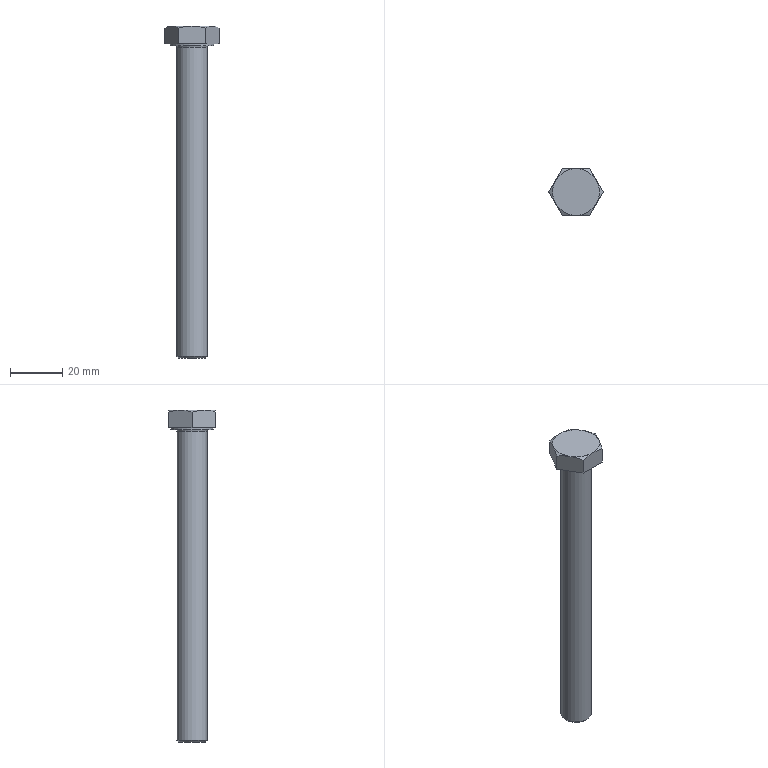Part | NX | features SKETCH 4, EXTRUDE 3, META 3, DATUM_CSYS 2, BLEND 1, CHAMFER 1, DATUM_PLANE 1, LINE 1, SWP104 1, SYMBOLIC_THREAD 1, THREADS 1 | 1 solid | 20 faces | box 20.785 x 18 x 127.5 mm | volume 15029 mm3 | plane 10 | cone 7 | cylinder 2 | torus 1 | commonest cylinder face diameters 11.732 x1 16.63 x1
STEP:
#1=CARTESIAN_POINT('',(5.196,-9.,6.696));
#2=VERTEX_POINT('',#1);
#3=CARTESIAN_POINT('',(7.794,-4.5,7.5));
#4=VERTEX_POINT('',#3);
#5=CARTESIAN_POINT('',(5.196,-9.,6.696));
#6=CARTESIAN_POINT('',(6.046,-7.528,7.187));
#7=CARTESIAN_POINT('',(6.909,-6.033,7.5));
#8=CARTESIAN_POINT('',(7.794,-4.5,7.5));
#9=B_SPLINE_CURVE_WITH_KNOTS('',3,(#5,#6,#7,#8),.UNSPECIFIED.,.F.,.F.,(4,4),(0.000000238,0.005258),.UNSPECIFIED.);
#10=EDGE_CURVE('',#2,#4,#9,.T.);
#11=ORIENTED_EDGE('',*,*,#10,.F.);
#12=CARTESIAN_POINT('',(5.196,-9.,0.6));
#13=VERTEX_POINT('',#12);
#14=CARTESIAN_POINT('',(5.196,-9.,7.5));
#15=DIRECTION('',(0.,0.,-1.));
#16=VECTOR('',#15,1000.);
#17=LINE('',#14,#16);
#18=EDGE_CURVE('',#2,#13,#17,.T.);
#19=ORIENTED_EDGE('',*,*,#18,.T.);
#20=CARTESIAN_POINT('',(10.392,0.,0.6));
#21=VERTEX_POINT('',#20);
#22=CARTESIAN_POINT('',(5.196,-9.,0.6));
#23=DIRECTION('',(0.5,0.866,0.));
#24=VECTOR('',#23,1000.);
#25=LINE('',#22,#24);
#26=EDGE_CURVE('',#13,#21,#25,.T.);
#27=ORIENTED_EDGE('',*,*,#26,.T.);
#28=CARTESIAN_POINT('',(10.392,0.,6.696));
#29=VERTEX_POINT('',#28);
#30=CARTESIAN_POINT('',(10.392,0.,7.5));
#31=DIRECTION('',(0.,0.,-1.));
#32=VECTOR('',#31,1000.);
#33=LINE('',#30,#32);
#34=EDGE_CURVE('',#29,#21,#33,.T.);
#35=ORIENTED_EDGE('',*,*,#34,.F.);
#36=CARTESIAN_POINT('',(7.794,-4.5,7.5));
#37=CARTESIAN_POINT('',(8.676,-2.972,7.5));
#38=CARTESIAN_POINT('',(9.544,-1.469,7.186));
#39=CARTESIAN_POINT('',(10.392,0.,6.696));
#40=B_SPLINE_CURVE_WITH_KNOTS('',3,(#36,#37,#38,#39),.UNSPECIFIED.,.F.,.F.,(4,4),(0.005258,0.0105),.UNSPECIFIED.);
#41=EDGE_CURVE('',#4,#29,#40,.T.);
#42=ORIENTED_EDGE('',*,*,#41,.F.);
#43=EDGE_LOOP('',(#11,#19,#27,#35,#42));
#44=FACE_BOUND('',#43,.T.);
#45=CARTESIAN_POINT('',(5.196,-9.,7.5));
#46=DIRECTION('',(-0.866,0.5,0.));
#47=DIRECTION('',(-0.5,-0.866,0.));
#48=AXIS2_PLACEMENT_3D('',#45,#46,#47);
#49=PLANE('',#48);
#50=ADVANCED_FACE('',(#44),#49,.F.);
#51=CARTESIAN_POINT('',(7.794,4.5,7.5));
#52=VERTEX_POINT('',#51);
#53=CARTESIAN_POINT('',(10.392,0.,6.696));
#54=CARTESIAN_POINT('',(9.542,1.472,7.187));
#55=CARTESIAN_POINT('',(8.679,2.967,7.5));
#56=CARTESIAN_POINT('',(7.794,4.5,7.5));
#57=B_SPLINE_CURVE_WITH_KNOTS('',3,(#53,#54,#55,#56),.UNSPECIFIED.,.F.,.F.,(4,4),(0.000000238,0.005258),.UNSPECIFIED.);
#58=EDGE_CURVE('',#29,#52,#57,.T.);
#59=ORIENTED_EDGE('',*,*,#58,.F.);
#60=ORIENTED_EDGE('',*,*,#34,.T.);
#61=CARTESIAN_POINT('',(5.196,9.,0.6));
#62=VERTEX_POINT('',#61);
#63=CARTESIAN_POINT('',(10.392,0.,0.6));
#64=DIRECTION('',(-0.5,0.866,0.));
#65=VECTOR('',#64,1000.);
#66=LINE('',#63,#65);
#67=EDGE_CURVE('',#21,#62,#66,.T.);
#68=ORIENTED_EDGE('',*,*,#67,.T.);
#69=CARTESIAN_POINT('',(5.196,9.,6.696));
#70=VERTEX_POINT('',#69);
#71=CARTESIAN_POINT('',(5.196,9.,7.5));
#72=DIRECTION('',(0.,0.,-1.));
#73=VECTOR('',#72,1000.);
#74=LINE('',#71,#73);
#75=EDGE_CURVE('',#70,#62,#74,.T.);
#76=ORIENTED_EDGE('',*,*,#75,.F.);
#77=CARTESIAN_POINT('',(7.794,4.5,7.5));
#78=CARTESIAN_POINT('',(6.912,6.028,7.5));
#79=CARTESIAN_POINT('',(6.044,7.531,7.186));
#80=CARTESIAN_POINT('',(5.196,9.,6.696));
#81=B_SPLINE_CURVE_WITH_KNOTS('',3,(#77,#78,#79,#80),.UNSPECIFIED.,.F.,.F.,(4,4),(0.005258,0.0105),.UNSPECIFIED.);
#82=EDGE_CURVE('',#52,#70,#81,.T.);
#83=ORIENTED_EDGE('',*,*,#82,.F.);
#84=EDGE_LOOP('',(#59,#60,#68,#76,#83));
#85=FACE_BOUND('',#84,.T.);
#86=CARTESIAN_POINT('',(10.392,0.,7.5));
#87=DIRECTION('',(-0.866,-0.5,0.));
#88=DIRECTION('',(0.5,-0.866,0.));
#89=AXIS2_PLACEMENT_3D('',#86,#87,#88);
#90=PLANE('',#89);
#91=ADVANCED_FACE('',(#85),#90,.F.);
#92=CARTESIAN_POINT('',(0.,9.,7.5));
#93=VERTEX_POINT('',#92);
#94=CARTESIAN_POINT('',(0.,9.,7.5));
#95=CARTESIAN_POINT('',(1.757,9.,7.5));
#96=CARTESIAN_POINT('',(3.516,9.,7.181));
#97=CARTESIAN_POINT('',(5.196,9.,6.696));
#98=B_SPLINE_CURVE_WITH_KNOTS('',3,(#94,#95,#96,#97),.UNSPECIFIED.,.F.,.F.,(4,4),(0.01453,0.01979),.UNSPECIFIED.);
#99=EDGE_CURVE('',#70,#93,#98,.F.);
#100=ORIENTED_EDGE('',*,*,#99,.F.);
#101=ORIENTED_EDGE('',*,*,#75,.T.);
#102=CARTESIAN_POINT('',(-5.196,9.,0.6));
#103=VERTEX_POINT('',#102);
#104=CARTESIAN_POINT('',(5.196,9.,0.6));
#105=DIRECTION('',(-1.,0.,0.));
#106=VECTOR('',#105,1000.);
#107=LINE('',#104,#106);
#108=EDGE_CURVE('',#62,#103,#107,.T.);
#109=ORIENTED_EDGE('',*,*,#108,.T.);
#110=CARTESIAN_POINT('',(-5.196,9.,6.696));
#111=VERTEX_POINT('',#110);
#112=CARTESIAN_POINT('',(-5.196,9.,7.5));
#113=DIRECTION('',(0.,0.,-1.));
#114=VECTOR('',#113,1000.);
#115=LINE('',#112,#114);
#116=EDGE_CURVE('',#111,#103,#115,.T.);
#117=ORIENTED_EDGE('',*,*,#116,.F.);
#118=CARTESIAN_POINT('',(-5.196,9.,6.696));
#119=CARTESIAN_POINT('',(-3.506,9.,7.184));
#120=CARTESIAN_POINT('',(-1.756,9.,7.5));
#121=CARTESIAN_POINT('',(0.,9.,7.5));
#122=B_SPLINE_CURVE_WITH_KNOTS('',3,(#118,#119,#120,#121),.UNSPECIFIED.,.F.,.F.,(4,4),(0.009271,0.01453),.UNSPECIFIED.);
#123=EDGE_CURVE('',#93,#111,#122,.F.);
#124=ORIENTED_EDGE('',*,*,#123,.F.);
#125=EDGE_LOOP('',(#100,#101,#109,#117,#124));
#126=FACE_BOUND('',#125,.T.);
#127=CARTESIAN_POINT('',(5.196,9.,7.5));
#128=DIRECTION('',(0.,-1.,0.));
#129=DIRECTION('',(0.,0.,-1.));
#130=AXIS2_PLACEMENT_3D('',#127,#128,#129);
#131=PLANE('',#130);
#132=ADVANCED_FACE('',(#126),#131,.F.);
#133=CARTESIAN_POINT('',(-7.794,4.5,7.5));
#134=VERTEX_POINT('',#133);
#135=CARTESIAN_POINT('',(-5.196,9.,6.696));
#136=CARTESIAN_POINT('',(-6.046,7.528,7.187));
#137=CARTESIAN_POINT('',(-6.909,6.033,7.5));
#138=CARTESIAN_POINT('',(-7.794,4.5,7.5));
#139=B_SPLINE_CURVE_WITH_KNOTS('',3,(#135,#136,#137,#138),.UNSPECIFIED.,.F.,.F.,(4,4),(0.000000238,0.005258),.UNSPECIFIED.);
#140=EDGE_CURVE('',#111,#134,#139,.T.);
#141=ORIENTED_EDGE('',*,*,#140,.F.);
#142=ORIENTED_EDGE('',*,*,#116,.T.);
#143=CARTESIAN_POINT('',(-10.392,0.,0.6));
#144=VERTEX_POINT('',#143);
#145=CARTESIAN_POINT('',(-5.196,9.,0.6));
#146=DIRECTION('',(-0.5,-0.866,0.));
#147=VECTOR('',#146,1000.);
#148=LINE('',#145,#147);
#149=EDGE_CURVE('',#103,#144,#148,.T.);
#150=ORIENTED_EDGE('',*,*,#149,.T.);
#151=CARTESIAN_POINT('',(-10.392,0.,6.696));
#152=VERTEX_POINT('',#151);
#153=CARTESIAN_POINT('',(-10.392,0.,7.5));
#154=DIRECTION('',(0.,0.,-1.));
#155=VECTOR('',#154,1000.);
#156=LINE('',#153,#155);
#157=EDGE_CURVE('',#152,#144,#156,.T.);
#158=ORIENTED_EDGE('',*,*,#157,.F.);
#159=CARTESIAN_POINT('',(-7.794,4.5,7.5));
#160=CARTESIAN_POINT('',(-8.676,2.972,7.5));
#161=CARTESIAN_POINT('',(-9.544,1.469,7.186));
#162=CARTESIAN_POINT('',(-10.392,0.,6.696));
#163=B_SPLINE_CURVE_WITH_KNOTS('',3,(#159,#160,#161,#162),.UNSPECIFIED.,.F.,.F.,(4,4),(0.005258,0.0105),.UNSPECIFIED.);
#164=EDGE_CURVE('',#134,#152,#163,.T.);
#165=ORIENTED_EDGE('',*,*,#164,.F.);
#166=EDGE_LOOP('',(#141,#142,#150,#158,#165));
#167=FACE_BOUND('',#166,.T.);
#168=CARTESIAN_POINT('',(-5.196,9.,7.5));
#169=DIRECTION('',(0.866,-0.5,0.));
#170=DIRECTION('',(0.5,0.866,0.));
#171=AXIS2_PLACEMENT_3D('',#168,#169,#170);
#172=PLANE('',#171);
#173=ADVANCED_FACE('',(#167),#172,.F.);
#174=CARTESIAN_POINT('',(-7.794,-4.5,7.5));
#175=VERTEX_POINT('',#174);
#176=CARTESIAN_POINT('',(-10.392,0.,6.696));
#177=CARTESIAN_POINT('',(-9.542,-1.472,7.187));
#178=CARTESIAN_POINT('',(-8.679,-2.967,7.5));
#179=CARTESIAN_POINT('',(-7.794,-4.5,7.5));
#180=B_SPLINE_CURVE_WITH_KNOTS('',3,(#176,#177,#178,#179),.UNSPECIFIED.,.F.,.F.,(4,4),(0.000000238,0.005258),.UNSPECIFIED.);
#181=EDGE_CURVE('',#152,#175,#180,.T.);
#182=ORIENTED_EDGE('',*,*,#181,.F.);
#183=ORIENTED_EDGE('',*,*,#157,.T.);
#184=CARTESIAN_POINT('',(-5.196,-9.,0.6));
#185=VERTEX_POINT('',#184);
#186=CARTESIAN_POINT('',(-10.392,0.,0.6));
#187=DIRECTION('',(0.5,-0.866,0.));
#188=VECTOR('',#187,1000.);
#189=LINE('',#186,#188);
#190=EDGE_CURVE('',#144,#185,#189,.T.);
#191=ORIENTED_EDGE('',*,*,#190,.T.);
#192=CARTESIAN_POINT('',(-5.196,-9.,6.696));
#193=VERTEX_POINT('',#192);
#194=CARTESIAN_POINT('',(-5.196,-9.,7.5));
#195=DIRECTION('',(0.,0.,-1.));
#196=VECTOR('',#195,1000.);
#197=LINE('',#194,#196);
#198=EDGE_CURVE('',#193,#185,#197,.T.);
#199=ORIENTED_EDGE('',*,*,#198,.F.);
#200=CARTESIAN_POINT('',(-7.794,-4.5,7.5));
#201=CARTESIAN_POINT('',(-6.912,-6.028,7.5));
#202=CARTESIAN_POINT('',(-6.044,-7.531,7.186));
#203=CARTESIAN_POINT('',(-5.196,-9.,6.696));
#204=B_SPLINE_CURVE_WITH_KNOTS('',3,(#200,#201,#202,#203),.UNSPECIFIED.,.F.,.F.,(4,4),(0.005258,0.0105),.UNSPECIFIED.);
#205=EDGE_CURVE('',#175,#193,#204,.T.);
#206=ORIENTED_EDGE('',*,*,#205,.F.);
#207=EDGE_LOOP('',(#182,#183,#191,#199,#206));
#208=FACE_BOUND('',#207,.T.);
#209=CARTESIAN_POINT('',(-10.392,0.,7.5));
#210=DIRECTION('',(0.866,0.5,0.));
#211=DIRECTION('',(-0.5,0.866,0.));
#212=AXIS2_PLACEMENT_3D('',#209,#210,#211);
#213=PLANE('',#212);
#214=ADVANCED_FACE('',(#208),#213,.F.);
#215=CARTESIAN_POINT('',(0.,-9.,7.5));
#216=VERTEX_POINT('',#215);
#217=CARTESIAN_POINT('',(-5.196,-9.,6.696));
#218=CARTESIAN_POINT('',(-3.506,-9.,7.184));
#219=CARTESIAN_POINT('',(-1.756,-9.,7.5));
#220=CARTESIAN_POINT('',(0.,-9.,7.5));
#221=B_SPLINE_CURVE_WITH_KNOTS('',3,(#217,#218,#219,#220),.UNSPECIFIED.,.F.,.F.,(4,4),(0.009271,0.01453),.UNSPECIFIED.);
#222=EDGE_CURVE('',#193,#216,#221,.T.);
#223=ORIENTED_EDGE('',*,*,#222,.F.);
#224=ORIENTED_EDGE('',*,*,#198,.T.);
#225=CARTESIAN_POINT('',(-5.196,-9.,0.6));
#226=DIRECTION('',(1.,0.,0.));
#227=VECTOR('',#226,1000.);
#228=LINE('',#225,#227);
#229=EDGE_CURVE('',#185,#13,#228,.T.);
#230=ORIENTED_EDGE('',*,*,#229,.T.);
#231=ORIENTED_EDGE('',*,*,#18,.F.);
#232=CARTESIAN_POINT('',(0.,-9.,7.5));
#233=CARTESIAN_POINT('',(1.757,-9.,7.5));
#234=CARTESIAN_POINT('',(3.516,-9.,7.181));
#235=CARTESIAN_POINT('',(5.196,-9.,6.696));
#236=B_SPLINE_CURVE_WITH_KNOTS('',3,(#232,#233,#234,#235),.UNSPECIFIED.,.F.,.F.,(4,4),(0.01453,0.01979),.UNSPECIFIED.);
#237=EDGE_CURVE('',#216,#2,#236,.T.);
#238=ORIENTED_EDGE('',*,*,#237,.F.);
#239=EDGE_LOOP('',(#223,#224,#230,#231,#238));
#240=FACE_BOUND('',#239,.T.);
#241=CARTESIAN_POINT('',(-5.196,-9.,7.5));
#242=DIRECTION('',(0.,1.,0.));
#243=DIRECTION('',(0.,0.,1.));
#244=AXIS2_PLACEMENT_3D('',#241,#242,#243);
#245=PLANE('',#244);
#246=ADVANCED_FACE('',(#240),#245,.F.);
#247=CARTESIAN_POINT('',(8.315,0.,0.6));
#248=VERTEX_POINT('',#247);
#249=CARTESIAN_POINT('',(0.,0.,0.6));
#250=DIRECTION('',(0.,0.,1.));
#251=DIRECTION('',(1.,0.,0.));
#252=AXIS2_PLACEMENT_3D('',#249,#250,#251);
#253=CIRCLE('',#252,8.315);
#254=EDGE_CURVE('',#248,#248,#253,.T.);
#255=ORIENTED_EDGE('',*,*,#254,.T.);
#256=EDGE_LOOP('',(#255));
#257=FACE_BOUND('',#256,.T.);
#258=ORIENTED_EDGE('',*,*,#26,.F.);
#259=ORIENTED_EDGE('',*,*,#229,.F.);
#260=ORIENTED_EDGE('',*,*,#190,.F.);
#261=ORIENTED_EDGE('',*,*,#149,.F.);
#262=ORIENTED_EDGE('',*,*,#108,.F.);
#263=ORIENTED_EDGE('',*,*,#67,.F.);
#264=EDGE_LOOP('',(#258,#259,#260,#261,#262,#263));
#265=FACE_BOUND('',#264,.T.);
#266=CARTESIAN_POINT('',(10.392,0.,0.6));
#267=DIRECTION('',(0.,0.,1.));
#268=DIRECTION('',(1.,0.,0.));
#269=AXIS2_PLACEMENT_3D('',#266,#267,#268);
#270=PLANE('',#269);
#271=ADVANCED_FACE('',(#257,#265),#270,.F.);
#272=ORIENTED_EDGE('',*,*,#10,.T.);
#273=CARTESIAN_POINT('',(0.,0.,7.5));
#274=DIRECTION('',(0.,0.,-1.));
#275=DIRECTION('',(-1.,0.,0.));
#276=AXIS2_PLACEMENT_3D('',#273,#274,#275);
#277=CIRCLE('',#276,9.);
#278=EDGE_CURVE('',#4,#216,#277,.T.);
#279=ORIENTED_EDGE('',*,*,#278,.T.);
#280=ORIENTED_EDGE('',*,*,#237,.T.);
#281=EDGE_LOOP('',(#272,#279,#280));
#282=FACE_BOUND('',#281,.T.);
#283=CARTESIAN_POINT('',(0.,0.,6.696));
#284=DIRECTION('',(0.,0.,-1.));
#285=DIRECTION('',(-1.,0.,0.));
#286=AXIS2_PLACEMENT_3D('',#283,#284,#285);
#287=CONICAL_SURFACE('',#286,10.392,1.047);
#288=ADVANCED_FACE('',(#282),#287,.T.);
#289=ORIENTED_EDGE('',*,*,#205,.T.);
#290=ORIENTED_EDGE('',*,*,#222,.T.);
#291=CARTESIAN_POINT('',(0.,0.,7.5));
#292=DIRECTION('',(0.,0.,-1.));
#293=DIRECTION('',(-1.,0.,0.));
#294=AXIS2_PLACEMENT_3D('',#291,#292,#293);
#295=CIRCLE('',#294,9.);
#296=EDGE_CURVE('',#216,#175,#295,.T.);
#297=ORIENTED_EDGE('',*,*,#296,.T.);
#298=EDGE_LOOP('',(#289,#290,#297));
#299=FACE_BOUND('',#298,.T.);
#300=CARTESIAN_POINT('',(0.,0.,6.696));
#301=DIRECTION('',(0.,0.,-1.));
#302=DIRECTION('',(-1.,0.,0.));
#303=AXIS2_PLACEMENT_3D('',#300,#301,#302);
#304=CONICAL_SURFACE('',#303,10.392,1.047);
#305=ADVANCED_FACE('',(#299),#304,.T.);
#306=ORIENTED_EDGE('',*,*,#164,.T.);
#307=ORIENTED_EDGE('',*,*,#181,.T.);
#308=CARTESIAN_POINT('',(0.,0.,7.5));
#309=DIRECTION('',(0.,0.,-1.));
#310=DIRECTION('',(-1.,0.,0.));
#311=AXIS2_PLACEMENT_3D('',#308,#309,#310);
#312=CIRCLE('',#311,9.);
#313=EDGE_CURVE('',#175,#134,#312,.T.);
#314=ORIENTED_EDGE('',*,*,#313,.T.);
#315=EDGE_LOOP('',(#306,#307,#314));
#316=FACE_BOUND('',#315,.T.);
#317=CARTESIAN_POINT('',(0.,0.,6.696));
#318=DIRECTION('',(0.,0.,-1.));
#319=DIRECTION('',(-1.,0.,0.));
#320=AXIS2_PLACEMENT_3D('',#317,#318,#319);
#321=CONICAL_SURFACE('',#320,10.392,1.047);
#322=ADVANCED_FACE('',(#316),#321,.T.);
#323=ORIENTED_EDGE('',*,*,#123,.T.);
#324=ORIENTED_EDGE('',*,*,#140,.T.);
#325=CARTESIAN_POINT('',(0.,0.,7.5));
#326=DIRECTION('',(0.,0.,-1.));
#327=DIRECTION('',(-1.,0.,0.));
#328=AXIS2_PLACEMENT_3D('',#325,#326,#327);
#329=CIRCLE('',#328,9.);
#330=EDGE_CURVE('',#134,#93,#329,.T.);
#331=ORIENTED_EDGE('',*,*,#330,.T.);
#332=EDGE_LOOP('',(#323,#324,#331));
#333=FACE_BOUND('',#332,.T.);
#334=CARTESIAN_POINT('',(0.,0.,6.696));
#335=DIRECTION('',(0.,0.,-1.));
#336=DIRECTION('',(-1.,0.,0.));
#337=AXIS2_PLACEMENT_3D('',#334,#335,#336);
#338=CONICAL_SURFACE('',#337,10.392,1.047);
#339=ADVANCED_FACE('',(#333),#338,.T.);
#340=ORIENTED_EDGE('',*,*,#82,.T.);
#341=ORIENTED_EDGE('',*,*,#99,.T.);
#342=CARTESIAN_POINT('',(0.,0.,7.5));
#343=DIRECTION('',(0.,0.,-1.));
#344=DIRECTION('',(-1.,0.,0.));
#345=AXIS2_PLACEMENT_3D('',#342,#343,#344);
#346=CIRCLE('',#345,9.);
#347=EDGE_CURVE('',#93,#52,#346,.T.);
#348=ORIENTED_EDGE('',*,*,#347,.T.);
#349=EDGE_LOOP('',(#340,#341,#348));
#350=FACE_BOUND('',#349,.T.);
#351=CARTESIAN_POINT('',(0.,0.,6.696));
#352=DIRECTION('',(0.,0.,-1.));
#353=DIRECTION('',(-1.,0.,0.));
#354=AXIS2_PLACEMENT_3D('',#351,#352,#353);
#355=CONICAL_SURFACE('',#354,10.392,1.047);
#356=ADVANCED_FACE('',(#350),#355,.T.);
#357=ORIENTED_EDGE('',*,*,#41,.T.);
#358=ORIENTED_EDGE('',*,*,#58,.T.);
#359=CARTESIAN_POINT('',(0.,0.,7.5));
#360=DIRECTION('',(0.,0.,-1.));
#361=DIRECTION('',(-1.,0.,0.));
#362=AXIS2_PLACEMENT_3D('',#359,#360,#361);
#363=CIRCLE('',#362,9.);
#364=EDGE_CURVE('',#52,#4,#363,.T.);
#365=ORIENTED_EDGE('',*,*,#364,.T.);
#366=EDGE_LOOP('',(#357,#358,#365));
#367=FACE_BOUND('',#366,.T.);
#368=CARTESIAN_POINT('',(0.,0.,6.696));
#369=DIRECTION('',(0.,0.,-1.));
#370=DIRECTION('',(-1.,0.,0.));
#371=AXIS2_PLACEMENT_3D('',#368,#369,#370);
#372=CONICAL_SURFACE('',#371,10.392,1.047);
#373=ADVANCED_FACE('',(#367),#372,.T.);
#374=ORIENTED_EDGE('',*,*,#330,.F.);
#375=ORIENTED_EDGE('',*,*,#313,.F.);
#376=ORIENTED_EDGE('',*,*,#296,.F.);
#377=ORIENTED_EDGE('',*,*,#278,.F.);
#378=ORIENTED_EDGE('',*,*,#364,.F.);
#379=ORIENTED_EDGE('',*,*,#347,.F.);
#380=EDGE_LOOP('',(#374,#375,#376,#377,#378,#379));
#381=FACE_BOUND('',#380,.T.);
#382=CARTESIAN_POINT('',(10.392,0.,7.5));
#383=DIRECTION('',(0.,0.,1.));
#384=DIRECTION('',(1.,0.,0.));
#385=AXIS2_PLACEMENT_3D('',#382,#383,#384);
#386=PLANE('',#385);
#387=ADVANCED_FACE('',(#381),#386,.T.);
#388=ORIENTED_EDGE('',*,*,#254,.F.);
#389=EDGE_LOOP('',(#388));
#390=FACE_BOUND('',#389,.T.);
#391=CARTESIAN_POINT('',(8.315,0.,0.));
#392=VERTEX_POINT('',#391);
#393=CARTESIAN_POINT('',(0.,0.,0.));
#394=DIRECTION('',(0.,0.,1.));
#395=DIRECTION('',(1.,0.,0.));
#396=AXIS2_PLACEMENT_3D('',#393,#394,#395);
#397=CIRCLE('',#396,8.315);
#398=EDGE_CURVE('',#392,#392,#397,.T.);
#399=ORIENTED_EDGE('',*,*,#398,.T.);
#400=EDGE_LOOP('',(#399));
#401=FACE_BOUND('',#400,.T.);
#402=CARTESIAN_POINT('',(0.,0.,0.6));
#403=DIRECTION('',(0.,0.,-1.));
#404=DIRECTION('',(-1.,0.,0.));
#405=AXIS2_PLACEMENT_3D('',#402,#403,#404);
#406=CYLINDRICAL_SURFACE('',#405,8.315);
#407=ADVANCED_FACE('',(#390,#401),#406,.T.);
#408=CARTESIAN_POINT('',(6.466,0.,0.));
#409=VERTEX_POINT('',#408);
#410=CARTESIAN_POINT('',(0.,0.,0.));
#411=DIRECTION('',(0.,0.,1.));
#412=DIRECTION('',(1.,0.,0.));
#413=AXIS2_PLACEMENT_3D('',#410,#411,#412);
#414=CIRCLE('',#413,6.466);
#415=EDGE_CURVE('',#409,#409,#414,.T.);
#416=ORIENTED_EDGE('',*,*,#415,.T.);
#417=EDGE_LOOP('',(#416));
#418=FACE_BOUND('',#417,.T.);
#419=ORIENTED_EDGE('',*,*,#398,.F.);
#420=EDGE_LOOP('',(#419));
#421=FACE_BOUND('',#420,.T.);
#422=CARTESIAN_POINT('',(0.,0.,0.));
#423=DIRECTION('',(0.,0.,1.));
#424=DIRECTION('',(1.,0.,0.));
#425=AXIS2_PLACEMENT_3D('',#422,#423,#424);
#426=PLANE('',#425);
#427=ADVANCED_FACE('',(#418,#421),#426,.F.);
#428=CARTESIAN_POINT('',(5.866,0.,-0.6));
#429=VERTEX_POINT('',#428);
#430=CARTESIAN_POINT('',(0.,0.,-0.6));
#431=DIRECTION('',(0.,0.,1.));
#432=DIRECTION('',(1.,0.,0.));
#433=AXIS2_PLACEMENT_3D('',#430,#431,#432);
#434=CIRCLE('',#433,5.866);
#435=EDGE_CURVE('',#429,#429,#434,.F.);
#436=ORIENTED_EDGE('',*,*,#435,.T.);
#437=EDGE_LOOP('',(#436));
#438=FACE_BOUND('',#437,.T.);
#439=CARTESIAN_POINT('',(5.866,0.,-119.413));
#440=VERTEX_POINT('',#439);
#441=CARTESIAN_POINT('',(0.,0.,-119.413));
#442=DIRECTION('',(0.,0.,1.));
#443=DIRECTION('',(1.,0.,0.));
#444=AXIS2_PLACEMENT_3D('',#441,#442,#443);
#445=CIRCLE('',#444,5.866);
#446=EDGE_CURVE('',#440,#440,#445,.T.);
#447=ORIENTED_EDGE('',*,*,#446,.T.);
#448=EDGE_LOOP('',(#447));
#449=FACE_BOUND('',#448,.T.);
#450=CARTESIAN_POINT('',(0.,0.,-120.));
#451=DIRECTION('',(0.,0.,1.));
#452=DIRECTION('',(1.,0.,0.));
#453=AXIS2_PLACEMENT_3D('',#450,#451,#452);
#454=CYLINDRICAL_SURFACE('',#453,5.866);
#455=ADVANCED_FACE('',(#438,#449),#454,.T.);
#456=CARTESIAN_POINT('',(5.279,0.,-120.));
#457=VERTEX_POINT('',#456);
#458=CARTESIAN_POINT('',(0.,0.,-120.));
#459=DIRECTION('',(0.,0.,1.));
#460=DIRECTION('',(1.,0.,0.));
#461=AXIS2_PLACEMENT_3D('',#458,#459,#460);
#462=CIRCLE('',#461,5.279);
#463=EDGE_CURVE('',#457,#457,#462,.F.);
#464=ORIENTED_EDGE('',*,*,#463,.T.);
#465=EDGE_LOOP('',(#464));
#466=FACE_BOUND('',#465,.T.);
#467=CARTESIAN_POINT('',(0.,0.,-120.));
#468=DIRECTION('',(0.,0.,1.));
#469=DIRECTION('',(1.,0.,0.));
#470=AXIS2_PLACEMENT_3D('',#467,#468,#469);
#471=PLANE('',#470);
#472=ADVANCED_FACE('',(#466),#471,.F.);
#473=ORIENTED_EDGE('',*,*,#463,.F.);
#474=EDGE_LOOP('',(#473));
#475=FACE_BOUND('',#474,.T.);
#476=ORIENTED_EDGE('',*,*,#446,.F.);
#477=EDGE_LOOP('',(#476));
#478=FACE_BOUND('',#477,.T.);
#479=CARTESIAN_POINT('',(0.,0.,-119.413));
#480=DIRECTION('',(0.,0.,1.));
#481=DIRECTION('',(1.,0.,0.));
#482=AXIS2_PLACEMENT_3D('',#479,#480,#481);
#483=CONICAL_SURFACE('',#482,5.866,0.7854);
#484=ADVANCED_FACE('',(#475,#478),#483,.T.);
#485=ORIENTED_EDGE('',*,*,#435,.F.);
#486=EDGE_LOOP('',(#485));
#487=FACE_BOUND('',#486,.T.);
#488=ORIENTED_EDGE('',*,*,#415,.F.);
#489=EDGE_LOOP('',(#488));
#490=FACE_BOUND('',#489,.T.);
#491=CARTESIAN_POINT('',(0.,0.,-0.6));
#492=DIRECTION('',(0.,0.,1.));
#493=DIRECTION('',(1.,0.,0.));
#494=AXIS2_PLACEMENT_3D('',#491,#492,#493);
#495=TOROIDAL_SURFACE('',#494,6.466,0.6);
#496=ADVANCED_FACE('',(#487,#490),#495,.F.);
#497=CLOSED_SHELL('',(#50,#91,#132,#173,#214,#246,#271,#288,#305,#322,#339,#356,#373,#387,#407,#427,#455,#472,#484,#496));
#498=MANIFOLD_SOLID_BREP('',#497);
#499=(LENGTH_UNIT()NAMED_UNIT(*)SI_UNIT(.MILLI.,.METRE.));
#500=UNCERTAINTY_MEASURE_WITH_UNIT(LENGTH_MEASURE(0.0508),#499,'','');
#501=(NAMED_UNIT(*)PLANE_ANGLE_UNIT()SI_UNIT($,.RADIAN.));
#502=(NAMED_UNIT(*)SI_UNIT($,.STERADIAN.)SOLID_ANGLE_UNIT());
#503=(GEOMETRIC_REPRESENTATION_CONTEXT(3)GLOBAL_UNCERTAINTY_ASSIGNED_CONTEXT((#500))GLOBAL_UNIT_ASSIGNED_CONTEXT((#499,#501,#502))REPRESENTATION_CONTEXT('',''));
#504=ADVANCED_BREP_SHAPE_REPRESENTATION('',(#498),#503);